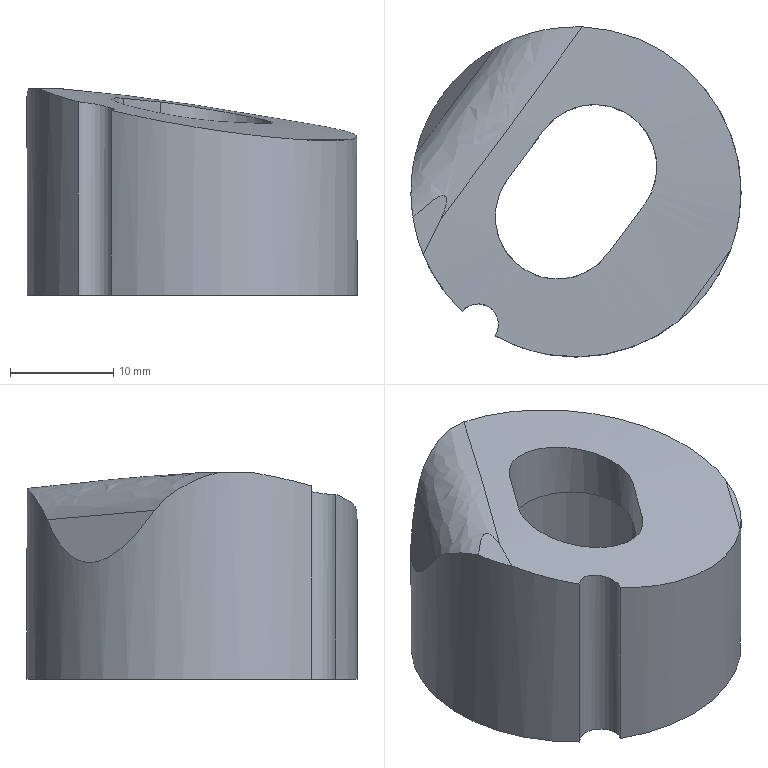Part | NX | features solid 2 | 1 solid | 14 faces | box 32.002 x 32 x 20.001 mm | volume 8892 mm3 | cylinder 5 | plane 5 | spline 4 | commonest cylinder face diameters 12.1 x2 4 x1 20.6 x1 32 x1
STEP:
#1=CARTESIAN_POINT('',(-895.514,283.241,15.738));
#2=VERTEX_POINT('',#1);
#3=CARTESIAN_POINT('',(-895.514,283.241,-3.));
#4=VERTEX_POINT('',#3);
#5=CARTESIAN_POINT('',(-895.514,283.241,7.));
#6=DIRECTION('',(0.,0.,1.));
#7=VECTOR('',#6,1000.);
#8=LINE('',#5,#7);
#9=EDGE_CURVE('',#2,#4,#8,.F.);
#10=ORIENTED_EDGE('',*,*,#9,.F.);
#11=CARTESIAN_POINT('',(-899.271,288.74,17.));
#12=VERTEX_POINT('',#11);
#13=CARTESIAN_POINT('',(-895.514,283.241,15.738));
#14=CARTESIAN_POINT('',(-897.14,284.792,16.198));
#15=CARTESIAN_POINT('',(-898.411,286.646,16.631));
#16=CARTESIAN_POINT('',(-899.271,288.74,17.));
#17=B_SPLINE_CURVE_WITH_KNOTS('',3,(#13,#14,#15,#16),.UNSPECIFIED.,.F.,.F.,(4,4),(0.,0.006783),.UNSPECIFIED.);
#18=EDGE_CURVE('',#2,#12,#17,.T.);
#19=ORIENTED_EDGE('',*,*,#18,.T.);
#20=CARTESIAN_POINT('',(-900.283,292.372,17.));
#21=VERTEX_POINT('',#20);
#22=CARTESIAN_POINT('',(-884.471,294.82,17.));
#23=DIRECTION('',(0.,0.,1.));
#24=DIRECTION('',(0.8041,-0.5945,0.));
#25=AXIS2_PLACEMENT_3D('',#22,#23,#24);
#26=CIRCLE('',#25,16.);
#27=EDGE_CURVE('',#21,#12,#26,.T.);
#28=ORIENTED_EDGE('',*,*,#27,.F.);
#29=CARTESIAN_POINT('',(-900.054,298.451,13.363));
#30=VERTEX_POINT('',#29);
#31=CARTESIAN_POINT('',(-900.054,298.451,13.364));
#32=CARTESIAN_POINT('',(-900.215,297.759,14.364));
#33=CARTESIAN_POINT('',(-900.552,295.786,15.797));
#34=CARTESIAN_POINT('',(-900.465,293.548,16.738));
#35=CARTESIAN_POINT('',(-900.283,292.372,17.));
#36=B_SPLINE_CURVE_WITH_KNOTS('',3,(#31,#32,#33,#34,#35),.UNSPECIFIED.,.F.,.F.,(4,1,4),(0.00005291,0.003662,0.007271),.UNSPECIFIED.);
#37=EDGE_CURVE('',#30,#21,#36,.T.);
#38=ORIENTED_EDGE('',*,*,#37,.F.);
#39=CARTESIAN_POINT('',(-892.21,308.824,12.452));
#40=VERTEX_POINT('',#39);
#41=CARTESIAN_POINT('',(-900.054,298.451,13.363));
#42=CARTESIAN_POINT('',(-899.869,299.241,12.221));
#43=CARTESIAN_POINT('',(-899.479,300.535,10.576));
#44=CARTESIAN_POINT('',(-898.519,302.555,8.915));
#45=CARTESIAN_POINT('',(-897.43,304.286,8.182));
#46=CARTESIAN_POINT('',(-896.043,305.932,8.408));
#47=CARTESIAN_POINT('',(-894.185,307.627,9.769));
#48=CARTESIAN_POINT('',(-892.968,308.405,11.341));
#49=CARTESIAN_POINT('',(-892.211,308.823,12.451));
#50=B_SPLINE_CURVE_WITH_KNOTS('',3,(#41,#42,#43,#44,#45,#46,#47,#48,#49),.UNSPECIFIED.,.F.,.F.,(4,1,1,1,1,1,4),(0.0003814,0.004577,0.006675,0.008773,0.01087,0.01297,0.01717),.UNSPECIFIED.);
#51=EDGE_CURVE('',#30,#40,#50,.T.);
#52=ORIENTED_EDGE('',*,*,#51,.T.);
#53=CARTESIAN_POINT('',(-883.852,310.808,15.384));
#54=VERTEX_POINT('',#53);
#55=CARTESIAN_POINT('',(-883.852,310.808,15.384));
#56=CARTESIAN_POINT('',(-885.432,310.869,15.657));
#57=CARTESIAN_POINT('',(-887.844,310.587,15.322));
#58=CARTESIAN_POINT('',(-890.602,309.649,14.029));
#59=CARTESIAN_POINT('',(-891.777,309.063,13.086));
#60=CARTESIAN_POINT('',(-892.209,308.824,12.452));
#61=B_SPLINE_CURVE_WITH_KNOTS('',3,(#55,#56,#57,#58,#59,#60),.UNSPECIFIED.,.F.,.F.,(4,1,1,4),(0.,0.00474,0.00711,0.00948),.UNSPECIFIED.);
#62=EDGE_CURVE('',#54,#40,#61,.T.);
#63=ORIENTED_EDGE('',*,*,#62,.F.);
#64=CARTESIAN_POINT('',(-869.466,289.266,12.058));
#65=VERTEX_POINT('',#64);
#66=CARTESIAN_POINT('',(-883.852,310.808,15.384));
#67=CARTESIAN_POINT('',(-881.365,310.711,14.956));
#68=CARTESIAN_POINT('',(-876.4,309.327,14.152));
#69=CARTESIAN_POINT('',(-870.701,304.091,13.225));
#70=CARTESIAN_POINT('',(-867.983,296.826,12.487));
#71=CARTESIAN_POINT('',(-868.587,291.647,12.148));
#72=CARTESIAN_POINT('',(-869.462,289.277,12.058));
#73=B_SPLINE_CURVE_WITH_KNOTS('',3,(#66,#67,#68,#69,#70,#71,#72),.UNSPECIFIED.,.F.,.F.,(4,1,1,1,4),(0.009525,0.01708,0.02464,0.03219,0.03975),.UNSPECIFIED.);
#74=EDGE_CURVE('',#54,#65,#73,.T.);
#75=ORIENTED_EDGE('',*,*,#74,.T.);
#76=CARTESIAN_POINT('',(-874.478,282.324,12.119));
#77=VERTEX_POINT('',#76);
#78=CARTESIAN_POINT('',(-869.467,289.262,12.058));
#79=CARTESIAN_POINT('',(-869.972,287.899,12.006));
#80=CARTESIAN_POINT('',(-871.325,285.364,11.905));
#81=CARTESIAN_POINT('',(-873.341,283.234,12.04));
#82=CARTESIAN_POINT('',(-874.475,282.327,12.118));
#83=B_SPLINE_CURVE_WITH_KNOTS('',3,(#78,#79,#80,#81,#82),.UNSPECIFIED.,.F.,.F.,(4,1,4),(0.,0.004301,0.008602),.UNSPECIFIED.);
#84=EDGE_CURVE('',#65,#77,#83,.T.);
#85=ORIENTED_EDGE('',*,*,#84,.T.);
#86=CARTESIAN_POINT('',(-892.304,280.868,14.91));
#87=VERTEX_POINT('',#86);
#88=CARTESIAN_POINT('',(-874.486,282.318,12.119));
#89=CARTESIAN_POINT('',(-876.987,280.32,12.293));
#90=CARTESIAN_POINT('',(-883.164,277.916,13.01));
#91=CARTESIAN_POINT('',(-889.551,279.322,14.258));
#92=CARTESIAN_POINT('',(-892.304,280.868,14.91));
#93=B_SPLINE_CURVE_WITH_KNOTS('',3,(#88,#89,#90,#91,#92),.UNSPECIFIED.,.F.,.F.,(4,1,4),(0.0484,0.05794,0.06748),.UNSPECIFIED.);
#94=EDGE_CURVE('',#77,#87,#93,.T.);
#95=ORIENTED_EDGE('',*,*,#94,.T.);
#96=CARTESIAN_POINT('',(-892.304,280.868,-3.));
#97=VERTEX_POINT('',#96);
#98=CARTESIAN_POINT('',(-892.304,280.868,7.));
#99=DIRECTION('',(0.,0.,1.));
#100=VECTOR('',#99,1000.);
#101=LINE('',#98,#100);
#102=EDGE_CURVE('',#97,#87,#101,.T.);
#103=ORIENTED_EDGE('',*,*,#102,.F.);
#104=CARTESIAN_POINT('',(-884.471,294.82,-3.));
#105=DIRECTION('',(0.,0.,1.));
#106=DIRECTION('',(0.8041,-0.5945,0.));
#107=AXIS2_PLACEMENT_3D('',#104,#105,#106);
#108=CIRCLE('',#107,16.);
#109=EDGE_CURVE('',#97,#4,#108,.T.);
#110=ORIENTED_EDGE('',*,*,#109,.T.);
#111=EDGE_LOOP('',(#10,#19,#28,#38,#52,#63,#75,#85,#95,#103,#110));
#112=FACE_BOUND('',#111,.T.);
#113=CARTESIAN_POINT('',(-884.471,294.82,-3.));
#114=DIRECTION('',(0.,0.,1.));
#115=DIRECTION('',(0.8041,-0.5945,0.));
#116=AXIS2_PLACEMENT_3D('',#113,#114,#115);
#117=CYLINDRICAL_SURFACE('',#116,16.);
#118=ADVANCED_FACE('',(#112),#117,.T.);
#119=CARTESIAN_POINT('',(-895.514,283.241,15.738));
#120=CARTESIAN_POINT('',(-895.184,283.634,15.721));
#121=CARTESIAN_POINT('',(-894.229,284.136,15.601));
#122=CARTESIAN_POINT('',(-892.684,283.722,15.28));
#123=CARTESIAN_POINT('',(-891.825,282.366,14.986));
#124=CARTESIAN_POINT('',(-892.025,281.299,14.908));
#125=CARTESIAN_POINT('',(-892.304,280.868,14.91));
#126=B_SPLINE_CURVE_WITH_KNOTS('',3,(#119,#120,#121,#122,#123,#124,#125),.UNSPECIFIED.,.F.,.F.,(4,1,1,1,4),(0.,0.001518,0.003036,0.004553,0.006071),.UNSPECIFIED.);
#127=EDGE_CURVE('',#2,#87,#126,.T.);
#128=ORIENTED_EDGE('',*,*,#127,.F.);
#129=ORIENTED_EDGE('',*,*,#9,.T.);
#130=CARTESIAN_POINT('',(-893.984,281.954,-3.));
#131=DIRECTION('',(0.,0.,1.));
#132=DIRECTION('',(-0.5945,-0.8041,0.));
#133=AXIS2_PLACEMENT_3D('',#130,#131,#132);
#134=CIRCLE('',#133,2.);
#135=EDGE_CURVE('',#97,#4,#134,.T.);
#136=ORIENTED_EDGE('',*,*,#135,.F.);
#137=ORIENTED_EDGE('',*,*,#102,.T.);
#138=EDGE_LOOP('',(#128,#129,#136,#137));
#139=FACE_BOUND('',#138,.T.);
#140=CARTESIAN_POINT('',(-893.984,281.954,-3.));
#141=DIRECTION('',(0.,0.,1.));
#142=DIRECTION('',(-0.5945,-0.8041,0.));
#143=AXIS2_PLACEMENT_3D('',#140,#141,#142);
#144=CYLINDRICAL_SURFACE('',#143,2.);
#145=ADVANCED_FACE('',(#139),#144,.F.);
#146=CARTESIAN_POINT('',(-891.119,296.004,16.081));
#147=VERTEX_POINT('',#146);
#148=CARTESIAN_POINT('',(-887.552,300.829,15.719));
#149=VERTEX_POINT('',#148);
#150=CARTESIAN_POINT('',(-891.119,296.004,16.081));
#151=CARTESIAN_POINT('',(-889.93,297.613,15.973));
#152=CARTESIAN_POINT('',(-888.741,299.221,15.851));
#153=CARTESIAN_POINT('',(-887.552,300.829,15.719));
#154=B_SPLINE_CURVE_WITH_KNOTS('',3,(#150,#151,#152,#153),.UNSPECIFIED.,.F.,.F.,(4,4),(0.,0.006011),.UNSPECIFIED.);
#155=EDGE_CURVE('',#147,#149,#154,.T.);
#156=ORIENTED_EDGE('',*,*,#155,.F.);
#157=CARTESIAN_POINT('',(-891.119,296.004,9.));
#158=VERTEX_POINT('',#157);
#159=CARTESIAN_POINT('',(-891.119,296.004,-3.));
#160=DIRECTION('',(0.,0.,1.));
#161=VECTOR('',#160,1000.);
#162=LINE('',#159,#161);
#163=EDGE_CURVE('',#158,#147,#162,.T.);
#164=ORIENTED_EDGE('',*,*,#163,.F.);
#165=CARTESIAN_POINT('',(-887.552,300.829,9.));
#166=VERTEX_POINT('',#165);
#167=CARTESIAN_POINT('',(-889.336,298.416,9.));
#168=DIRECTION('',(-0.5945,-0.8041,0.));
#169=VECTOR('',#168,1000.);
#170=LINE('',#167,#169);
#171=EDGE_CURVE('',#166,#158,#170,.T.);
#172=ORIENTED_EDGE('',*,*,#171,.F.);
#173=CARTESIAN_POINT('',(-887.552,300.829,-3.));
#174=DIRECTION('',(0.,0.,1.));
#175=VECTOR('',#174,1000.);
#176=LINE('',#173,#175);
#177=EDGE_CURVE('',#166,#149,#176,.T.);
#178=ORIENTED_EDGE('',*,*,#177,.T.);
#179=EDGE_LOOP('',(#156,#164,#172,#178));
#180=FACE_BOUND('',#179,.T.);
#181=CARTESIAN_POINT('',(-887.552,300.829,-3.));
#182=DIRECTION('',(-0.8041,0.5945,0.));
#183=DIRECTION('',(0.,0.,1.));
#184=AXIS2_PLACEMENT_3D('',#181,#182,#183);
#185=PLANE('',#184);
#186=ADVANCED_FACE('',(#180),#185,.F.);
#187=CARTESIAN_POINT('',(-881.39,288.81,13.806));
#188=VERTEX_POINT('',#187);
#189=CARTESIAN_POINT('',(-888.385,286.745,14.817));
#190=VERTEX_POINT('',#189);
#191=CARTESIAN_POINT('',(-881.39,288.81,13.806));
#192=CARTESIAN_POINT('',(-882.181,287.741,13.844));
#193=CARTESIAN_POINT('',(-884.447,286.183,14.078));
#194=CARTESIAN_POINT('',(-887.172,286.288,14.56));
#195=CARTESIAN_POINT('',(-888.385,286.745,14.817));
#196=B_SPLINE_CURVE_WITH_KNOTS('',3,(#191,#192,#193,#194,#195),.UNSPECIFIED.,.F.,.F.,(4,1,4),(0.,0.003933,0.007866),.UNSPECIFIED.);
#197=EDGE_CURVE('',#188,#190,#196,.T.);
#198=ORIENTED_EDGE('',*,*,#197,.F.);
#199=CARTESIAN_POINT('',(-881.39,288.81,9.));
#200=VERTEX_POINT('',#199);
#201=CARTESIAN_POINT('',(-881.39,288.81,-3.));
#202=DIRECTION('',(0.,0.,1.));
#203=VECTOR('',#202,1000.);
#204=LINE('',#201,#203);
#205=EDGE_CURVE('',#200,#188,#204,.T.);
#206=ORIENTED_EDGE('',*,*,#205,.F.);
#207=CARTESIAN_POINT('',(-886.255,292.407,9.));
#208=DIRECTION('',(0.,0.,1.));
#209=DIRECTION('',(0.8041,-0.5945,0.));
#210=AXIS2_PLACEMENT_3D('',#207,#208,#209);
#211=CIRCLE('',#210,6.05);
#212=EDGE_CURVE('',#158,#200,#211,.T.);
#213=ORIENTED_EDGE('',*,*,#212,.F.);
#214=ORIENTED_EDGE('',*,*,#163,.T.);
#215=CARTESIAN_POINT('',(-892.001,290.513,15.811));
#216=VERTEX_POINT('',#215);
#217=CARTESIAN_POINT('',(-892.001,290.513,15.811));
#218=CARTESIAN_POINT('',(-892.596,292.318,16.078));
#219=CARTESIAN_POINT('',(-892.277,294.439,16.187));
#220=CARTESIAN_POINT('',(-891.119,296.004,16.081));
#221=B_SPLINE_CURVE_WITH_KNOTS('',3,(#217,#218,#219,#220),.UNSPECIFIED.,.F.,.F.,(4,4),(0.01333,0.0191),.UNSPECIFIED.);
#222=EDGE_CURVE('',#216,#147,#221,.T.);
#223=ORIENTED_EDGE('',*,*,#222,.F.);
#224=CARTESIAN_POINT('',(-888.385,286.745,14.817));
#225=CARTESIAN_POINT('',(-889.1,287.014,14.968));
#226=CARTESIAN_POINT('',(-890.195,287.727,15.223));
#227=CARTESIAN_POINT('',(-890.817,288.423,15.404));
#228=CARTESIAN_POINT('',(-891.055,288.723,15.477));
#229=CARTESIAN_POINT('',(-891.141,288.839,15.504));
#230=CARTESIAN_POINT('',(-891.167,288.875,15.512));
#231=CARTESIAN_POINT('',(-891.286,289.044,15.549));
#232=CARTESIAN_POINT('',(-891.522,289.414,15.626));
#233=CARTESIAN_POINT('',(-891.778,289.91,15.717));
#234=CARTESIAN_POINT('',(-891.935,290.315,15.781));
#235=CARTESIAN_POINT('',(-892.001,290.513,15.811));
#236=B_SPLINE_CURVE_WITH_KNOTS('',3,(#224,#225,#226,#227,#228,#229,#230,#231,#232,#233,#234,#235),.UNSPECIFIED.,.F.,.F.,(4,1,1,1,1,1,1,1,1,4),(0.,0.25,0.5,0.5625,0.625,0.6562,0.6875,0.75,0.875,1.),.UNSPECIFIED.);
#237=EDGE_CURVE('',#190,#216,#236,.T.);
#238=ORIENTED_EDGE('',*,*,#237,.F.);
#239=EDGE_LOOP('',(#198,#206,#213,#214,#223,#238));
#240=FACE_BOUND('',#239,.T.);
#241=CARTESIAN_POINT('',(-886.255,292.407,-3.));
#242=DIRECTION('',(0.,0.,1.));
#243=DIRECTION('',(0.8041,-0.5945,0.));
#244=AXIS2_PLACEMENT_3D('',#241,#242,#243);
#245=CYLINDRICAL_SURFACE('',#244,6.05);
#246=ADVANCED_FACE('',(#240),#245,.F.);
#247=ORIENTED_EDGE('',*,*,#205,.T.);
#248=CARTESIAN_POINT('',(-877.823,293.635,13.62));
#249=VERTEX_POINT('',#248);
#250=CARTESIAN_POINT('',(-881.39,288.81,13.806));
#251=CARTESIAN_POINT('',(-880.201,290.419,13.749));
#252=CARTESIAN_POINT('',(-879.012,292.027,13.687));
#253=CARTESIAN_POINT('',(-877.823,293.635,13.62));
#254=B_SPLINE_CURVE_WITH_KNOTS('',3,(#250,#251,#252,#253),.UNSPECIFIED.,.F.,.F.,(4,4),(0.,0.006003),.UNSPECIFIED.);
#255=EDGE_CURVE('',#188,#249,#254,.T.);
#256=ORIENTED_EDGE('',*,*,#255,.T.);
#257=CARTESIAN_POINT('',(-877.823,293.635,9.));
#258=VERTEX_POINT('',#257);
#259=CARTESIAN_POINT('',(-877.823,293.635,-3.));
#260=DIRECTION('',(0.,0.,1.));
#261=VECTOR('',#260,1000.);
#262=LINE('',#259,#261);
#263=EDGE_CURVE('',#258,#249,#262,.T.);
#264=ORIENTED_EDGE('',*,*,#263,.F.);
#265=CARTESIAN_POINT('',(-879.607,291.223,9.));
#266=DIRECTION('',(-0.5945,-0.8041,0.));
#267=VECTOR('',#266,1000.);
#268=LINE('',#265,#267);
#269=EDGE_CURVE('',#258,#200,#268,.T.);
#270=ORIENTED_EDGE('',*,*,#269,.T.);
#271=EDGE_LOOP('',(#247,#256,#264,#270));
#272=FACE_BOUND('',#271,.T.);
#273=CARTESIAN_POINT('',(-877.823,293.635,-3.));
#274=DIRECTION('',(-0.8041,0.5945,0.));
#275=DIRECTION('',(0.,0.,1.));
#276=AXIS2_PLACEMENT_3D('',#273,#274,#275);
#277=PLANE('',#276);
#278=ADVANCED_FACE('',(#272),#277,.T.);
#279=CARTESIAN_POINT('',(-880.292,302.786,14.561));
#280=VERTEX_POINT('',#279);
#281=CARTESIAN_POINT('',(-887.552,300.829,15.719));
#282=CARTESIAN_POINT('',(-886.733,301.936,15.628));
#283=CARTESIAN_POINT('',(-884.362,303.523,15.27));
#284=CARTESIAN_POINT('',(-881.539,303.325,14.787));
#285=CARTESIAN_POINT('',(-880.291,302.787,14.561));
#286=B_SPLINE_CURVE_WITH_KNOTS('',3,(#281,#282,#283,#284,#285),.UNSPECIFIED.,.F.,.F.,(4,1,4),(0.,0.004081,0.008162),.UNSPECIFIED.);
#287=EDGE_CURVE('',#149,#280,#286,.T.);
#288=ORIENTED_EDGE('',*,*,#287,.F.);
#289=ORIENTED_EDGE('',*,*,#177,.F.);
#290=CARTESIAN_POINT('',(-882.688,297.232,9.));
#291=DIRECTION('',(0.,0.,1.));
#292=DIRECTION('',(0.8041,-0.5945,0.));
#293=AXIS2_PLACEMENT_3D('',#290,#291,#292);
#294=CIRCLE('',#293,6.05);
#295=EDGE_CURVE('',#258,#166,#294,.T.);
#296=ORIENTED_EDGE('',*,*,#295,.F.);
#297=ORIENTED_EDGE('',*,*,#263,.T.);
#298=CARTESIAN_POINT('',(-877.689,300.655,14.044));
#299=VERTEX_POINT('',#298);
#300=CARTESIAN_POINT('',(-877.696,300.65,14.045));
#301=CARTESIAN_POINT('',(-876.999,299.632,13.884));
#302=CARTESIAN_POINT('',(-876.241,297.124,13.625));
#303=CARTESIAN_POINT('',(-877.073,294.649,13.578));
#304=CARTESIAN_POINT('',(-877.823,293.635,13.62));
#305=B_SPLINE_CURVE_WITH_KNOTS('',3,(#300,#301,#302,#303,#304),.UNSPECIFIED.,.F.,.F.,(4,1,4),(0.01159,0.01532,0.01906),.UNSPECIFIED.);
#306=EDGE_CURVE('',#299,#249,#305,.T.);
#307=ORIENTED_EDGE('',*,*,#306,.F.);
#308=CARTESIAN_POINT('',(-880.291,302.787,14.561));
#309=CARTESIAN_POINT('',(-879.102,302.274,14.345));
#310=CARTESIAN_POINT('',(-878.247,301.455,14.173));
#311=CARTESIAN_POINT('',(-877.696,300.65,14.045));
#312=B_SPLINE_CURVE_WITH_KNOTS('',3,(#308,#309,#310,#311),.UNSPECIFIED.,.F.,.F.,(4,4),(0.,1.),.UNSPECIFIED.);
#313=EDGE_CURVE('',#280,#299,#312,.T.);
#314=ORIENTED_EDGE('',*,*,#313,.F.);
#315=EDGE_LOOP('',(#288,#289,#296,#297,#307,#314));
#316=FACE_BOUND('',#315,.T.);
#317=CARTESIAN_POINT('',(-882.688,297.232,-3.));
#318=DIRECTION('',(0.,0.,1.));
#319=DIRECTION('',(0.8041,-0.5945,0.));
#320=AXIS2_PLACEMENT_3D('',#317,#318,#319);
#321=CYLINDRICAL_SURFACE('',#320,6.05);
#322=ADVANCED_FACE('',(#316),#321,.F.);
#323=CARTESIAN_POINT('',(-876.189,288.696,-3.));
#324=VERTEX_POINT('',#323);
#325=CARTESIAN_POINT('',(-884.471,294.82,-3.));
#326=DIRECTION('',(0.,0.,1.));
#327=DIRECTION('',(0.8041,-0.5945,0.));
#328=AXIS2_PLACEMENT_3D('',#325,#326,#327);
#329=CIRCLE('',#328,10.3);
#330=EDGE_CURVE('',#324,#324,#329,.T.);
#331=ORIENTED_EDGE('',*,*,#330,.T.);
#332=EDGE_LOOP('',(#331));
#333=FACE_BOUND('',#332,.T.);
#334=ORIENTED_EDGE('',*,*,#109,.F.);
#335=ORIENTED_EDGE('',*,*,#135,.T.);
#336=EDGE_LOOP('',(#334,#335));
#337=FACE_BOUND('',#336,.T.);
#338=CARTESIAN_POINT('',(-884.471,294.82,-3.));
#339=DIRECTION('',(0.,0.,1.));
#340=DIRECTION('',(0.8041,-0.5945,0.));
#341=AXIS2_PLACEMENT_3D('',#338,#339,#340);
#342=PLANE('',#341);
#343=ADVANCED_FACE('',(#333,#337),#342,.F.);
#344=CARTESIAN_POINT('',(-897.597,292.138,17.));
#345=VERTEX_POINT('',#344);
#346=CARTESIAN_POINT('',(-900.283,292.372,17.));
#347=CARTESIAN_POINT('',(-899.906,292.726,17.));
#348=CARTESIAN_POINT('',(-899.329,293.246,17.));
#349=CARTESIAN_POINT('',(-898.514,293.889,17.));
#350=CARTESIAN_POINT('',(-897.967,294.237,17.));
#351=CARTESIAN_POINT('',(-897.497,294.458,17.));
#352=CARTESIAN_POINT('',(-897.042,294.425,17.));
#353=CARTESIAN_POINT('',(-896.984,293.97,17.));
#354=CARTESIAN_POINT('',(-897.075,293.471,17.));
#355=CARTESIAN_POINT('',(-897.282,292.85,17.));
#356=CARTESIAN_POINT('',(-897.488,292.374,17.));
#357=CARTESIAN_POINT('',(-897.597,292.137,17.));
#358=B_SPLINE_CURVE_WITH_KNOTS('',3,(#346,#347,#348,#349,#350,#351,#352,#353,#354,#355,#356,#357),.UNSPECIFIED.,.F.,.F.,(4,1,1,1,1,1,1,1,1,4),(0.004738,0.006289,0.007064,0.00784,0.008227,0.008615,0.009003,0.00939,0.01017,0.01094),.UNSPECIFIED.);
#359=EDGE_CURVE('',#21,#345,#358,.T.);
#360=ORIENTED_EDGE('',*,*,#359,.F.);
#361=ORIENTED_EDGE('',*,*,#27,.T.);
#362=CARTESIAN_POINT('',(-899.271,288.74,17.));
#363=CARTESIAN_POINT('',(-898.681,289.86,17.));
#364=CARTESIAN_POINT('',(-898.122,290.992,17.));
#365=CARTESIAN_POINT('',(-897.597,292.137,17.));
#366=B_SPLINE_CURVE_WITH_KNOTS('',3,(#362,#363,#364,#365),.UNSPECIFIED.,.F.,.F.,(4,4),(0.002381,0.006155),.UNSPECIFIED.);
#367=EDGE_CURVE('',#12,#345,#366,.T.);
#368=ORIENTED_EDGE('',*,*,#367,.T.);
#369=EDGE_LOOP('',(#360,#361,#368));
#370=FACE_BOUND('',#369,.T.);
#371=CARTESIAN_POINT('',(-884.471,294.82,17.));
#372=DIRECTION('',(0.,0.,1.));
#373=DIRECTION('',(0.8041,-0.5945,0.));
#374=AXIS2_PLACEMENT_3D('',#371,#372,#373);
#375=PLANE('',#374);
#376=ADVANCED_FACE('',(#370),#375,.T.);
#377=ORIENTED_EDGE('',*,*,#330,.F.);
#378=EDGE_LOOP('',(#377));
#379=FACE_BOUND('',#378,.T.);
#380=CARTESIAN_POINT('',(-876.189,288.696,9.));
#381=VERTEX_POINT('',#380);
#382=CARTESIAN_POINT('',(-884.471,294.82,9.));
#383=DIRECTION('',(0.,0.,1.));
#384=DIRECTION('',(0.8041,-0.5945,0.));
#385=AXIS2_PLACEMENT_3D('',#382,#383,#384);
#386=CIRCLE('',#385,10.3);
#387=EDGE_CURVE('',#381,#381,#386,.T.);
#388=ORIENTED_EDGE('',*,*,#387,.T.);
#389=EDGE_LOOP('',(#388));
#390=FACE_BOUND('',#389,.T.);
#391=CARTESIAN_POINT('',(-884.471,294.82,-3.));
#392=DIRECTION('',(0.,0.,1.));
#393=DIRECTION('',(0.8041,-0.5945,0.));
#394=AXIS2_PLACEMENT_3D('',#391,#392,#393);
#395=CYLINDRICAL_SURFACE('',#394,10.3);
#396=ADVANCED_FACE('',(#379,#390),#395,.F.);
#397=ORIENTED_EDGE('',*,*,#295,.T.);
#398=ORIENTED_EDGE('',*,*,#171,.T.);
#399=ORIENTED_EDGE('',*,*,#212,.T.);
#400=ORIENTED_EDGE('',*,*,#269,.F.);
#401=EDGE_LOOP('',(#397,#398,#399,#400));
#402=FACE_BOUND('',#401,.T.);
#403=ORIENTED_EDGE('',*,*,#387,.F.);
#404=EDGE_LOOP('',(#403));
#405=FACE_BOUND('',#404,.T.);
#406=CARTESIAN_POINT('',(-884.471,294.82,9.));
#407=DIRECTION('',(0.,0.,1.));
#408=DIRECTION('',(0.8041,-0.5945,0.));
#409=AXIS2_PLACEMENT_3D('',#406,#407,#408);
#410=PLANE('',#409);
#411=ADVANCED_FACE('',(#402,#405),#410,.F.);
#412=CARTESIAN_POINT('',(-883.852,310.808,15.384));
#413=CARTESIAN_POINT('',(-885.189,308.954,15.592));
#414=CARTESIAN_POINT('',(-887.153,306.246,15.878));
#415=CARTESIAN_POINT('',(-889.687,302.779,16.209));
#416=CARTESIAN_POINT('',(-891.545,300.252,16.431));
#417=CARTESIAN_POINT('',(-893.061,298.203,16.595));
#418=CARTESIAN_POINT('',(-894.246,296.608,16.713));
#419=CARTESIAN_POINT('',(-894.993,295.607,16.783));
#420=CARTESIAN_POINT('',(-895.55,294.861,16.833));
#421=CARTESIAN_POINT('',(-895.976,294.292,16.87));
#422=CARTESIAN_POINT('',(-896.094,294.135,16.88));
#423=CARTESIAN_POINT('',(-896.257,293.917,16.894));
#424=CARTESIAN_POINT('',(-896.538,293.544,16.917));
#425=CARTESIAN_POINT('',(-896.989,292.946,16.954));
#426=CARTESIAN_POINT('',(-897.389,292.418,16.985));
#427=CARTESIAN_POINT('',(-897.6,292.14,17.001));
#428=B_SPLINE_CURVE_WITH_KNOTS('',3,(#412,#413,#414,#415,#416,#417,#418,#419,#420,#421,#422,#423,#424,#425,#426,#427),.UNSPECIFIED.,.F.,.F.,(4,1,1,1,1,1,1,1,1,1,1,1,1,4),(0.3861,0.4212,0.4388,0.4563,0.4739,0.4827,0.4915,0.4959,0.5003,0.5025,0.5047,0.5091,0.5178,0.5266),.UNSPECIFIED.);
#429=EDGE_CURVE('',#54,#345,#428,.T.);
#430=ORIENTED_EDGE('',*,*,#429,.T.);
#431=ORIENTED_EDGE('',*,*,#367,.F.);
#432=ORIENTED_EDGE('',*,*,#18,.F.);
#433=ORIENTED_EDGE('',*,*,#127,.T.);
#434=ORIENTED_EDGE('',*,*,#94,.F.);
#435=CARTESIAN_POINT('',(-874.482,282.323,12.119));
#436=CARTESIAN_POINT('',(-872.815,284.62,12.099));
#437=CARTESIAN_POINT('',(-871.143,286.936,12.078));
#438=CARTESIAN_POINT('',(-869.466,289.271,12.058));
#439=B_SPLINE_CURVE_WITH_KNOTS('',3,(#435,#436,#437,#438),.UNSPECIFIED.,.F.,.F.,(4,4),(0.8352,0.9009),.UNSPECIFIED.);
#440=EDGE_CURVE('',#77,#65,#439,.T.);
#441=ORIENTED_EDGE('',*,*,#440,.T.);
#442=ORIENTED_EDGE('',*,*,#74,.F.);
#443=EDGE_LOOP('',(#430,#431,#432,#433,#434,#441,#442));
#444=FACE_BOUND('',#443,.T.);
#445=ORIENTED_EDGE('',*,*,#287,.T.);
#446=ORIENTED_EDGE('',*,*,#313,.T.);
#447=ORIENTED_EDGE('',*,*,#306,.T.);
#448=ORIENTED_EDGE('',*,*,#255,.F.);
#449=ORIENTED_EDGE('',*,*,#197,.T.);
#450=ORIENTED_EDGE('',*,*,#237,.T.);
#451=ORIENTED_EDGE('',*,*,#222,.T.);
#452=ORIENTED_EDGE('',*,*,#155,.T.);
#453=EDGE_LOOP('',(#445,#446,#447,#448,#449,#450,#451,#452));
#454=FACE_BOUND('',#453,.T.);
#455=CARTESIAN_POINT('',(-881.127,272.651,12.127));
#456=CARTESIAN_POINT('',(-882.862,273.89,12.543));
#457=CARTESIAN_POINT('',(-884.597,275.129,12.964));
#458=CARTESIAN_POINT('',(-886.332,276.368,13.389));
#459=CARTESIAN_POINT('',(-890.379,279.257,14.393));
#460=CARTESIAN_POINT('',(-894.424,282.146,15.42));
#461=CARTESIAN_POINT('',(-896.735,283.796,16.015));
#462=CARTESIAN_POINT('',(-899.045,285.446,16.616));
#463=CARTESIAN_POINT('',(-901.355,287.095,17.222));
#464=CARTESIAN_POINT('',(-881.025,272.794,12.127));
#465=CARTESIAN_POINT('',(-882.76,274.033,12.542));
#466=CARTESIAN_POINT('',(-884.496,275.272,12.963));
#467=CARTESIAN_POINT('',(-886.23,276.51,13.388));
#468=CARTESIAN_POINT('',(-890.277,279.4,14.391));
#469=CARTESIAN_POINT('',(-894.323,282.288,15.417));
#470=CARTESIAN_POINT('',(-896.633,283.939,16.012));
#471=CARTESIAN_POINT('',(-898.944,285.588,16.613));
#472=CARTESIAN_POINT('',(-901.254,287.238,17.218));
#473=CARTESIAN_POINT('',(-880.923,272.936,12.126));
#474=CARTESIAN_POINT('',(-882.659,274.175,12.542));
#475=CARTESIAN_POINT('',(-884.394,275.414,12.962));
#476=CARTESIAN_POINT('',(-886.129,276.653,13.386));
#477=CARTESIAN_POINT('',(-890.176,279.543,14.389));
#478=CARTESIAN_POINT('',(-894.221,282.431,15.415));
#479=CARTESIAN_POINT('',(-896.532,284.081,16.008));
#480=CARTESIAN_POINT('',(-898.842,285.731,16.609));
#481=CARTESIAN_POINT('',(-901.152,287.381,17.214));
#482=CARTESIAN_POINT('',(-880.822,273.079,12.126));
#483=CARTESIAN_POINT('',(-882.557,274.318,12.541));
#484=CARTESIAN_POINT('',(-884.293,275.557,12.961));
#485=CARTESIAN_POINT('',(-886.027,276.795,13.385));
#486=CARTESIAN_POINT('',(-890.075,279.685,14.386));
#487=CARTESIAN_POINT('',(-894.12,282.574,15.412));
#488=CARTESIAN_POINT('',(-896.431,284.224,16.005));
#489=CARTESIAN_POINT('',(-898.741,285.874,16.606));
#490=CARTESIAN_POINT('',(-901.051,287.523,17.21));
#491=CARTESIAN_POINT('',(-879.472,274.972,12.121));
#492=CARTESIAN_POINT('',(-881.208,276.211,12.531));
#493=CARTESIAN_POINT('',(-882.944,277.451,12.946));
#494=CARTESIAN_POINT('',(-884.679,278.689,13.366));
#495=CARTESIAN_POINT('',(-888.727,281.58,14.357));
#496=CARTESIAN_POINT('',(-892.773,284.469,15.373));
#497=CARTESIAN_POINT('',(-895.084,286.119,15.962));
#498=CARTESIAN_POINT('',(-897.395,287.769,16.557));
#499=CARTESIAN_POINT('',(-899.706,289.419,17.155));
#500=CARTESIAN_POINT('',(-878.123,276.865,12.114));
#501=CARTESIAN_POINT('',(-879.859,278.105,12.517));
#502=CARTESIAN_POINT('',(-881.595,279.344,12.927));
#503=CARTESIAN_POINT('',(-883.331,280.584,13.341));
#504=CARTESIAN_POINT('',(-887.38,283.475,14.32));
#505=CARTESIAN_POINT('',(-891.427,286.364,15.324));
#506=CARTESIAN_POINT('',(-893.739,288.015,15.906));
#507=CARTESIAN_POINT('',(-896.05,289.666,16.492));
#508=CARTESIAN_POINT('',(-898.362,291.316,17.082));
#509=CARTESIAN_POINT('',(-876.875,278.616,12.105));
#510=CARTESIAN_POINT('',(-878.612,279.856,12.503));
#511=CARTESIAN_POINT('',(-880.349,281.096,12.905));
#512=CARTESIAN_POINT('',(-882.085,282.336,13.313));
#513=CARTESIAN_POINT('',(-886.135,285.227,14.278));
#514=CARTESIAN_POINT('',(-890.183,288.118,15.268));
#515=CARTESIAN_POINT('',(-892.496,289.769,15.84));
#516=CARTESIAN_POINT('',(-894.808,291.42,16.417));
#517=CARTESIAN_POINT('',(-897.12,293.071,16.999));
#518=CARTESIAN_POINT('',(-874.406,282.082,12.085));
#519=CARTESIAN_POINT('',(-876.144,283.323,12.467));
#520=CARTESIAN_POINT('',(-877.882,284.563,12.855));
#521=CARTESIAN_POINT('',(-879.62,285.804,13.249));
#522=CARTESIAN_POINT('',(-883.673,288.697,14.179));
#523=CARTESIAN_POINT('',(-887.724,291.589,15.134));
#524=CARTESIAN_POINT('',(-890.038,293.242,15.686));
#525=CARTESIAN_POINT('',(-892.352,294.894,16.242));
#526=CARTESIAN_POINT('',(-894.666,296.546,16.803));
#527=CARTESIAN_POINT('',(-871.937,285.547,12.061));
#528=CARTESIAN_POINT('',(-873.677,286.789,12.423));
#529=CARTESIAN_POINT('',(-875.416,288.031,12.792));
#530=CARTESIAN_POINT('',(-877.156,289.272,13.167));
#531=CARTESIAN_POINT('',(-881.212,292.168,14.052));
#532=CARTESIAN_POINT('',(-885.267,295.063,14.961));
#533=CARTESIAN_POINT('',(-887.584,296.717,15.486));
#534=CARTESIAN_POINT('',(-889.901,298.371,16.016));
#535=CARTESIAN_POINT('',(-892.216,300.024,16.55));
#536=CARTESIAN_POINT('',(-870.715,287.262,12.049));
#537=CARTESIAN_POINT('',(-872.456,288.505,12.401));
#538=CARTESIAN_POINT('',(-874.197,289.747,12.759));
#539=CARTESIAN_POINT('',(-875.937,290.989,13.122));
#540=CARTESIAN_POINT('',(-879.996,293.886,13.983));
#541=CARTESIAN_POINT('',(-884.053,296.782,14.866));
#542=CARTESIAN_POINT('',(-886.371,298.437,15.377));
#543=CARTESIAN_POINT('',(-888.688,300.091,15.892));
#544=CARTESIAN_POINT('',(-891.006,301.746,16.411));
#545=CARTESIAN_POINT('',(-868.306,290.645,12.025));
#546=CARTESIAN_POINT('',(-870.049,291.889,12.354));
#547=CARTESIAN_POINT('',(-871.791,293.132,12.689));
#548=CARTESIAN_POINT('',(-873.533,294.375,13.029));
#549=CARTESIAN_POINT('',(-877.597,297.276,13.834));
#550=CARTESIAN_POINT('',(-881.659,300.175,14.662));
#551=CARTESIAN_POINT('',(-883.979,301.831,15.142));
#552=CARTESIAN_POINT('',(-886.299,303.487,15.626));
#553=CARTESIAN_POINT('',(-888.619,305.143,16.113));
#554=CARTESIAN_POINT('',(-865.896,294.028,11.999));
#555=CARTESIAN_POINT('',(-867.641,295.273,12.302));
#556=CARTESIAN_POINT('',(-869.386,296.518,12.61));
#557=CARTESIAN_POINT('',(-871.13,297.762,12.924));
#558=CARTESIAN_POINT('',(-875.199,300.666,13.665));
#559=CARTESIAN_POINT('',(-879.267,303.569,14.429));
#560=CARTESIAN_POINT('',(-881.59,305.227,14.872));
#561=CARTESIAN_POINT('',(-883.914,306.885,15.319));
#562=CARTESIAN_POINT('',(-886.237,308.543,15.771));
#563=CARTESIAN_POINT('',(-864.708,295.696,11.987));
#564=CARTESIAN_POINT('',(-866.455,296.942,12.276));
#565=CARTESIAN_POINT('',(-868.2,298.187,12.57));
#566=CARTESIAN_POINT('',(-869.946,299.433,12.869));
#567=CARTESIAN_POINT('',(-874.018,302.338,13.577));
#568=CARTESIAN_POINT('',(-878.088,305.242,14.308));
#569=CARTESIAN_POINT('',(-880.413,306.902,14.731));
#570=CARTESIAN_POINT('',(-882.738,308.561,15.16));
#571=CARTESIAN_POINT('',(-885.063,310.22,15.592));
#572=CARTESIAN_POINT('',(-863.52,297.364,11.973));
#573=CARTESIAN_POINT('',(-865.268,298.61,12.248));
#574=CARTESIAN_POINT('',(-867.015,299.857,12.527));
#575=CARTESIAN_POINT('',(-868.762,301.103,12.811));
#576=CARTESIAN_POINT('',(-872.836,304.01,13.485));
#577=CARTESIAN_POINT('',(-876.909,306.917,14.181));
#578=CARTESIAN_POINT('',(-879.236,308.577,14.584));
#579=CARTESIAN_POINT('',(-881.563,310.237,14.992));
#580=CARTESIAN_POINT('',(-883.889,311.897,15.405));
#581=CARTESIAN_POINT('',(-862.332,299.032,11.959));
#582=CARTESIAN_POINT('',(-864.081,300.279,12.219));
#583=CARTESIAN_POINT('',(-865.829,301.526,12.483));
#584=CARTESIAN_POINT('',(-867.577,302.774,12.752));
#585=CARTESIAN_POINT('',(-871.655,305.683,13.39));
#586=CARTESIAN_POINT('',(-875.731,308.591,14.048));
#587=CARTESIAN_POINT('',(-878.06,310.252,14.43));
#588=CARTESIAN_POINT('',(-880.389,311.914,14.818));
#589=CARTESIAN_POINT('',(-882.717,313.575,15.209));
#590=B_SPLINE_SURFACE_WITH_KNOTS('',5,5,((#455,#456,#457,#458,#459,#460,#461,#462,#463),(#464,#465,#466,#467,#468,#469,#470,#471,#472),(#473,#474,#475,#476,#477,#478,#479,#480,#481),(#482,#483,#484,#485,#486,#487,#488,#489,#490),(#491,#492,#493,#494,#495,#496,#497,#498,#499),(#500,#501,#502,#503,#504,#505,#506,#507,#508),(#509,#510,#511,#512,#513,#514,#515,#516,#517),(#518,#519,#520,#521,#522,#523,#524,#525,#526),(#527,#528,#529,#530,#531,#532,#533,#534,#535),(#536,#537,#538,#539,#540,#541,#542,#543,#544),(#545,#546,#547,#548,#549,#550,#551,#552,#553),(#554,#555,#556,#557,#558,#559,#560,#561,#562),(#563,#564,#565,#566,#567,#568,#569,#570,#571),(#572,#573,#574,#575,#576,#577,#578,#579,#580),(#581,#582,#583,#584,#585,#586,#587,#588,#589)),.UNSPECIFIED.,.F.,.F.,.F.,(6,3,3,3,6),(6,3,6),(0.6499,0.6529,0.69,0.7264,0.7618),(0.3047,0.518,0.8025),.UNSPECIFIED.);
#591=ADVANCED_FACE('',(#444,#454),#590,.T.);
#592=ORIENTED_EDGE('',*,*,#440,.F.);
#593=ORIENTED_EDGE('',*,*,#84,.F.);
#594=EDGE_LOOP('',(#592,#593));
#595=FACE_BOUND('',#594,.T.);
#596=CARTESIAN_POINT('',(-869.433,289.31,12.057));
#597=CARTESIAN_POINT('',(-869.316,289.224,12.034));
#598=CARTESIAN_POINT('',(-869.199,289.138,12.007));
#599=CARTESIAN_POINT('',(-869.083,289.052,11.976));
#600=CARTESIAN_POINT('',(-868.968,288.968,11.941));
#601=CARTESIAN_POINT('',(-868.854,288.883,11.902));
#602=CARTESIAN_POINT('',(-869.853,288.725,12.062));
#603=CARTESIAN_POINT('',(-869.736,288.639,12.039));
#604=CARTESIAN_POINT('',(-869.619,288.553,12.012));
#605=CARTESIAN_POINT('',(-869.503,288.467,11.98));
#606=CARTESIAN_POINT('',(-869.388,288.383,11.945));
#607=CARTESIAN_POINT('',(-869.274,288.298,11.906));
#608=CARTESIAN_POINT('',(-870.273,288.14,12.067));
#609=CARTESIAN_POINT('',(-870.156,288.054,12.043));
#610=CARTESIAN_POINT('',(-870.04,287.968,12.016));
#611=CARTESIAN_POINT('',(-869.924,287.883,11.984));
#612=CARTESIAN_POINT('',(-869.809,287.798,11.949));
#613=CARTESIAN_POINT('',(-869.695,287.714,11.91));
#614=CARTESIAN_POINT('',(-870.694,287.555,12.072));
#615=CARTESIAN_POINT('',(-870.577,287.469,12.048));
#616=CARTESIAN_POINT('',(-870.461,287.383,12.02));
#617=CARTESIAN_POINT('',(-870.345,287.298,11.989));
#618=CARTESIAN_POINT('',(-870.23,287.213,11.953));
#619=CARTESIAN_POINT('',(-870.116,287.129,11.914));
#620=CARTESIAN_POINT('',(-871.707,286.148,12.084));
#621=CARTESIAN_POINT('',(-871.591,286.062,12.06));
#622=CARTESIAN_POINT('',(-871.475,285.977,12.031));
#623=CARTESIAN_POINT('',(-871.36,285.891,11.999));
#624=CARTESIAN_POINT('',(-871.245,285.807,11.963));
#625=CARTESIAN_POINT('',(-871.132,285.723,11.923));
#626=CARTESIAN_POINT('',(-872.723,284.743,12.097));
#627=CARTESIAN_POINT('',(-872.607,284.657,12.072));
#628=CARTESIAN_POINT('',(-872.491,284.571,12.043));
#629=CARTESIAN_POINT('',(-872.376,284.486,12.01));
#630=CARTESIAN_POINT('',(-872.262,284.402,11.974));
#631=CARTESIAN_POINT('',(-872.149,284.318,11.933));
#632=CARTESIAN_POINT('',(-873.317,283.921,12.104));
#633=CARTESIAN_POINT('',(-873.201,283.835,12.079));
#634=CARTESIAN_POINT('',(-873.086,283.75,12.05));
#635=CARTESIAN_POINT('',(-872.971,283.665,12.017));
#636=CARTESIAN_POINT('',(-872.857,283.581,11.98));
#637=CARTESIAN_POINT('',(-872.744,283.497,11.94));
#638=CARTESIAN_POINT('',(-873.913,283.1,12.111));
#639=CARTESIAN_POINT('',(-873.797,283.014,12.086));
#640=CARTESIAN_POINT('',(-873.682,282.929,12.057));
#641=CARTESIAN_POINT('',(-873.567,282.844,12.024));
#642=CARTESIAN_POINT('',(-873.453,282.76,11.987));
#643=CARTESIAN_POINT('',(-873.34,282.676,11.946));
#644=CARTESIAN_POINT('',(-874.509,282.28,12.119));
#645=CARTESIAN_POINT('',(-874.393,282.194,12.093));
#646=CARTESIAN_POINT('',(-874.278,282.109,12.064));
#647=CARTESIAN_POINT('',(-874.164,282.024,12.03));
#648=CARTESIAN_POINT('',(-874.05,281.939,11.993));
#649=CARTESIAN_POINT('',(-873.937,281.856,11.952));
#650=B_SPLINE_SURFACE_WITH_KNOTS('',5,5,((#596,#597,#598,#599,#600,#601),(#602,#603,#604,#605,#606,#607),(#608,#609,#610,#611,#612,#613),(#614,#615,#616,#617,#618,#619),(#620,#621,#622,#623,#624,#625),(#626,#627,#628,#629,#630,#631),(#632,#633,#634,#635,#636,#637),(#638,#639,#640,#641,#642,#643),(#644,#645,#646,#647,#648,#649)),.UNSPECIFIED.,.F.,.F.,.F.,(6,3,6),(6,6),(0.1002,0.1278,0.1666),(0.,0.1212),.UNSPECIFIED.);
#651=ADVANCED_FACE('',(#595),#650,.T.);
#652=ORIENTED_EDGE('',*,*,#62,.T.);
#653=CARTESIAN_POINT('',(-900.054,298.451,13.364));
#654=CARTESIAN_POINT('',(-897.431,301.892,13.123));
#655=CARTESIAN_POINT('',(-894.817,305.351,12.814));
#656=CARTESIAN_POINT('',(-892.21,308.823,12.452));
#657=B_SPLINE_CURVE_WITH_KNOTS('',3,(#653,#654,#655,#656),.UNSPECIFIED.,.F.,.F.,(4,4),(0.5075,0.5797),.UNSPECIFIED.);
#658=EDGE_CURVE('',#30,#40,#657,.T.);
#659=ORIENTED_EDGE('',*,*,#658,.F.);
#660=ORIENTED_EDGE('',*,*,#37,.T.);
#661=ORIENTED_EDGE('',*,*,#359,.T.);
#662=ORIENTED_EDGE('',*,*,#429,.F.);
#663=EDGE_LOOP('',(#652,#659,#660,#661,#662));
#664=FACE_BOUND('',#663,.T.);
#665=CARTESIAN_POINT('',(-883.766,310.927,15.371));
#666=CARTESIAN_POINT('',(-884.323,311.356,15.471));
#667=CARTESIAN_POINT('',(-884.902,311.785,15.448));
#668=CARTESIAN_POINT('',(-885.478,312.198,15.296));
#669=CARTESIAN_POINT('',(-886.577,312.955,14.748));
#670=CARTESIAN_POINT('',(-887.482,313.518,13.777));
#671=CARTESIAN_POINT('',(-887.865,313.737,13.201));
#672=CARTESIAN_POINT('',(-888.162,313.885,12.561));
#673=CARTESIAN_POINT('',(-888.365,313.957,11.884));
#674=CARTESIAN_POINT('',(-888.367,313.958,11.876));
#675=CARTESIAN_POINT('',(-888.369,313.959,11.868));
#676=CARTESIAN_POINT('',(-888.372,313.96,11.86));
#677=CARTESIAN_POINT('',(-888.374,313.961,11.852));
#678=CARTESIAN_POINT('',(-888.377,313.961,11.843));
#679=CARTESIAN_POINT('',(-884.243,310.265,15.445));
#680=CARTESIAN_POINT('',(-884.801,310.694,15.548));
#681=CARTESIAN_POINT('',(-885.381,311.125,15.526));
#682=CARTESIAN_POINT('',(-885.958,311.54,15.375));
#683=CARTESIAN_POINT('',(-887.059,312.3,14.828));
#684=CARTESIAN_POINT('',(-887.966,312.866,13.856));
#685=CARTESIAN_POINT('',(-888.35,313.086,13.28));
#686=CARTESIAN_POINT('',(-888.647,313.235,12.638));
#687=CARTESIAN_POINT('',(-888.849,313.308,11.96));
#688=CARTESIAN_POINT('',(-888.852,313.309,11.952));
#689=CARTESIAN_POINT('',(-888.854,313.31,11.944));
#690=CARTESIAN_POINT('',(-888.857,313.311,11.936));
#691=CARTESIAN_POINT('',(-888.859,313.312,11.927));
#692=CARTESIAN_POINT('',(-888.862,313.312,11.919));
#693=CARTESIAN_POINT('',(-884.721,309.604,15.518));
#694=CARTESIAN_POINT('',(-885.28,310.034,15.623));
#695=CARTESIAN_POINT('',(-885.86,310.466,15.603));
#696=CARTESIAN_POINT('',(-886.439,310.882,15.453));
#697=CARTESIAN_POINT('',(-887.542,311.645,14.907));
#698=CARTESIAN_POINT('',(-888.45,312.214,13.934));
#699=CARTESIAN_POINT('',(-888.835,312.436,13.357));
#700=CARTESIAN_POINT('',(-889.132,312.585,12.714));
#701=CARTESIAN_POINT('',(-889.335,312.659,12.035));
#702=CARTESIAN_POINT('',(-889.337,312.66,12.026));
#703=CARTESIAN_POINT('',(-889.34,312.661,12.018));
#704=CARTESIAN_POINT('',(-889.342,312.662,12.01));
#705=CARTESIAN_POINT('',(-889.344,312.663,12.002));
#706=CARTESIAN_POINT('',(-889.347,312.664,11.994));
#707=CARTESIAN_POINT('',(-885.199,308.942,15.59));
#708=CARTESIAN_POINT('',(-885.759,309.373,15.697));
#709=CARTESIAN_POINT('',(-886.34,309.806,15.678));
#710=CARTESIAN_POINT('',(-886.92,310.223,15.53));
#711=CARTESIAN_POINT('',(-888.025,310.989,14.985));
#712=CARTESIAN_POINT('',(-888.935,311.561,14.011));
#713=CARTESIAN_POINT('',(-889.32,311.785,13.433));
#714=CARTESIAN_POINT('',(-889.618,311.935,12.789));
#715=CARTESIAN_POINT('',(-889.82,312.01,12.108));
#716=CARTESIAN_POINT('',(-889.823,312.011,12.1));
#717=CARTESIAN_POINT('',(-889.825,312.012,12.092));
#718=CARTESIAN_POINT('',(-889.827,312.013,12.084));
#719=CARTESIAN_POINT('',(-889.83,312.014,12.075));
#720=CARTESIAN_POINT('',(-889.832,312.015,12.067));
#721=CARTESIAN_POINT('',(-887.78,305.378,15.97));
#722=CARTESIAN_POINT('',(-888.343,305.813,16.088));
#723=CARTESIAN_POINT('',(-888.93,306.253,16.078));
#724=CARTESIAN_POINT('',(-889.515,306.678,15.935));
#725=CARTESIAN_POINT('',(-890.631,307.46,15.397));
#726=CARTESIAN_POINT('',(-891.549,308.049,14.418));
#727=CARTESIAN_POINT('',(-891.937,308.28,13.835));
#728=CARTESIAN_POINT('',(-892.235,308.437,13.184));
#729=CARTESIAN_POINT('',(-892.436,308.517,12.497));
#730=CARTESIAN_POINT('',(-892.439,308.517,12.488));
#731=CARTESIAN_POINT('',(-892.441,308.518,12.48));
#732=CARTESIAN_POINT('',(-892.444,308.519,12.472));
#733=CARTESIAN_POINT('',(-892.446,308.52,12.464));
#734=CARTESIAN_POINT('',(-892.448,308.521,12.455));
#735=CARTESIAN_POINT('',(-890.377,301.825,16.31));
#736=CARTESIAN_POINT('',(-890.942,302.264,16.438));
#737=CARTESIAN_POINT('',(-891.532,302.709,16.436));
#738=CARTESIAN_POINT('',(-892.122,303.141,16.298));
#739=CARTESIAN_POINT('',(-893.246,303.94,15.765));
#740=CARTESIAN_POINT('',(-894.17,304.545,14.782));
#741=CARTESIAN_POINT('',(-894.559,304.784,14.195));
#742=CARTESIAN_POINT('',(-894.857,304.948,13.539));
#743=CARTESIAN_POINT('',(-895.057,305.034,12.845));
#744=CARTESIAN_POINT('',(-895.059,305.035,12.836));
#745=CARTESIAN_POINT('',(-895.061,305.036,12.828));
#746=CARTESIAN_POINT('',(-895.064,305.037,12.82));
#747=CARTESIAN_POINT('',(-895.066,305.038,12.811));
#748=CARTESIAN_POINT('',(-895.069,305.039,12.803));
#749=CARTESIAN_POINT('',(-892.503,298.94,16.555));
#750=CARTESIAN_POINT('',(-893.071,299.381,16.69));
#751=CARTESIAN_POINT('',(-893.664,299.83,16.694));
#752=CARTESIAN_POINT('',(-894.256,300.268,16.56));
#753=CARTESIAN_POINT('',(-895.385,301.079,16.031));
#754=CARTESIAN_POINT('',(-896.311,301.698,15.045));
#755=CARTESIAN_POINT('',(-896.7,301.944,14.455));
#756=CARTESIAN_POINT('',(-896.998,302.114,13.795));
#757=CARTESIAN_POINT('',(-897.195,302.205,13.096));
#758=CARTESIAN_POINT('',(-897.197,302.206,13.088));
#759=CARTESIAN_POINT('',(-897.199,302.207,13.079));
#760=CARTESIAN_POINT('',(-897.202,302.208,13.071));
#761=CARTESIAN_POINT('',(-897.204,302.209,13.063));
#762=CARTESIAN_POINT('',(-897.207,302.21,13.054));
#763=CARTESIAN_POINT('',(-894.992,295.595,16.8));
#764=CARTESIAN_POINT('',(-895.561,296.039,16.942));
#765=CARTESIAN_POINT('',(-896.156,296.493,16.951));
#766=CARTESIAN_POINT('',(-896.751,296.936,16.822));
#767=CARTESIAN_POINT('',(-897.883,297.761,16.296));
#768=CARTESIAN_POINT('',(-898.81,298.396,15.308));
#769=CARTESIAN_POINT('',(-899.199,298.649,14.714));
#770=CARTESIAN_POINT('',(-899.494,298.826,14.05));
#771=CARTESIAN_POINT('',(-899.688,298.923,13.347));
#772=CARTESIAN_POINT('',(-899.691,298.924,13.339));
#773=CARTESIAN_POINT('',(-899.693,298.925,13.33));
#774=CARTESIAN_POINT('',(-899.695,298.927,13.322));
#775=CARTESIAN_POINT('',(-899.698,298.928,13.313));
#776=CARTESIAN_POINT('',(-899.7,298.929,13.305));
#777=CARTESIAN_POINT('',(-897.497,292.267,16.993));
#778=CARTESIAN_POINT('',(-898.068,292.713,17.141));
#779=CARTESIAN_POINT('',(-898.664,293.17,17.154));
#780=CARTESIAN_POINT('',(-899.26,293.619,17.028));
#781=CARTESIAN_POINT('',(-900.394,294.456,16.505));
#782=CARTESIAN_POINT('',(-901.319,295.106,15.514));
#783=CARTESIAN_POINT('',(-901.706,295.367,14.919));
#784=CARTESIAN_POINT('',(-901.998,295.552,14.252));
#785=CARTESIAN_POINT('',(-902.188,295.656,13.545));
#786=CARTESIAN_POINT('',(-902.191,295.657,13.536));
#787=CARTESIAN_POINT('',(-902.193,295.658,13.528));
#788=CARTESIAN_POINT('',(-902.195,295.659,13.519));
#789=CARTESIAN_POINT('',(-902.198,295.661,13.511));
#790=CARTESIAN_POINT('',(-902.2,295.662,13.502));
#791=CARTESIAN_POINT('',(-897.85,291.799,17.019));
#792=CARTESIAN_POINT('',(-898.421,292.245,17.167));
#793=CARTESIAN_POINT('',(-899.018,292.703,17.182));
#794=CARTESIAN_POINT('',(-899.613,293.153,17.056));
#795=CARTESIAN_POINT('',(-900.748,293.992,16.534));
#796=CARTESIAN_POINT('',(-901.672,294.644,15.542));
#797=CARTESIAN_POINT('',(-902.059,294.906,14.946));
#798=CARTESIAN_POINT('',(-902.351,295.091,14.279));
#799=CARTESIAN_POINT('',(-902.54,295.196,13.572));
#800=CARTESIAN_POINT('',(-902.543,295.197,13.563));
#801=CARTESIAN_POINT('',(-902.545,295.199,13.555));
#802=CARTESIAN_POINT('',(-902.547,295.2,13.546));
#803=CARTESIAN_POINT('',(-902.55,295.201,13.538));
#804=CARTESIAN_POINT('',(-902.552,295.202,13.529));
#805=CARTESIAN_POINT('',(-898.203,291.331,17.044));
#806=CARTESIAN_POINT('',(-898.774,291.778,17.193));
#807=CARTESIAN_POINT('',(-899.371,292.236,17.208));
#808=CARTESIAN_POINT('',(-899.967,292.686,17.082));
#809=CARTESIAN_POINT('',(-901.101,293.527,16.561));
#810=CARTESIAN_POINT('',(-902.026,294.181,15.569));
#811=CARTESIAN_POINT('',(-902.412,294.444,14.973));
#812=CARTESIAN_POINT('',(-902.704,294.631,14.305));
#813=CARTESIAN_POINT('',(-902.893,294.737,13.597));
#814=CARTESIAN_POINT('',(-902.895,294.738,13.589));
#815=CARTESIAN_POINT('',(-902.897,294.739,13.58));
#816=CARTESIAN_POINT('',(-902.899,294.741,13.572));
#817=CARTESIAN_POINT('',(-902.902,294.742,13.563));
#818=CARTESIAN_POINT('',(-902.904,294.743,13.555));
#819=CARTESIAN_POINT('',(-898.557,290.864,17.068));
#820=CARTESIAN_POINT('',(-899.128,291.311,17.218));
#821=CARTESIAN_POINT('',(-899.725,291.77,17.234));
#822=CARTESIAN_POINT('',(-900.321,292.22,17.108));
#823=CARTESIAN_POINT('',(-901.455,293.063,16.587));
#824=CARTESIAN_POINT('',(-902.379,293.719,15.595));
#825=CARTESIAN_POINT('',(-902.765,293.984,14.998));
#826=CARTESIAN_POINT('',(-903.056,294.171,14.33));
#827=CARTESIAN_POINT('',(-903.245,294.278,13.622));
#828=CARTESIAN_POINT('',(-903.247,294.279,13.613));
#829=CARTESIAN_POINT('',(-903.249,294.281,13.605));
#830=CARTESIAN_POINT('',(-903.252,294.282,13.596));
#831=CARTESIAN_POINT('',(-903.254,294.283,13.588));
#832=CARTESIAN_POINT('',(-903.256,294.284,13.579));
#833=B_SPLINE_SURFACE_WITH_KNOTS('',5,5,((#665,#666,#667,#668,#669,#670,#671,#672,#673,#674,#675,#676,#677,#678),(#679,#680,#681,#682,#683,#684,#685,#686,#687,#688,#689,#690,#691,#692),(#693,#694,#695,#696,#697,#698,#699,#700,#701,#702,#703,#704,#705,#706),(#707,#708,#709,#710,#711,#712,#713,#714,#715,#716,#717,#718,#719,#720),(#721,#722,#723,#724,#725,#726,#727,#728,#729,#730,#731,#732,#733,#734),(#735,#736,#737,#738,#739,#740,#741,#742,#743,#744,#745,#746,#747,#748),(#749,#750,#751,#752,#753,#754,#755,#756,#757,#758,#759,#760,#761,#762),(#763,#764,#765,#766,#767,#768,#769,#770,#771,#772,#773,#774,#775,#776),(#777,#778,#779,#780,#781,#782,#783,#784,#785,#786,#787,#788,#789,#790),(#791,#792,#793,#794,#795,#796,#797,#798,#799,#800,#801,#802,#803,#804),(#805,#806,#807,#808,#809,#810,#811,#812,#813,#814,#815,#816,#817,#818),(#819,#820,#821,#822,#823,#824,#825,#826,#827,#828,#829,#830,#831,#832)),.UNSPECIFIED.,.F.,.F.,.F.,(6,3,3,6),(6,3,5,6),(0.3849,0.4074,0.5058,0.5219),(0.,0.497,0.994,1.),.UNSPECIFIED.);
#834=ADVANCED_FACE('',(#664),#833,.F.);
#835=ORIENTED_EDGE('',*,*,#658,.T.);
#836=ORIENTED_EDGE('',*,*,#51,.F.);
#837=EDGE_LOOP('',(#835,#836));
#838=FACE_BOUND('',#837,.T.);
#839=CARTESIAN_POINT('',(-900.089,298.384,13.409));
#840=CARTESIAN_POINT('',(-900.091,298.385,13.403));
#841=CARTESIAN_POINT('',(-900.092,298.386,13.397));
#842=CARTESIAN_POINT('',(-900.094,298.386,13.391));
#843=CARTESIAN_POINT('',(-900.096,298.387,13.385));
#844=CARTESIAN_POINT('',(-900.098,298.387,13.379));
#845=CARTESIAN_POINT('',(-900.385,298.485,12.433));
#846=CARTESIAN_POINT('',(-900.671,298.583,11.487));
#847=CARTESIAN_POINT('',(-900.956,298.681,10.54));
#848=CARTESIAN_POINT('',(-901.24,298.779,9.592));
#849=CARTESIAN_POINT('',(-901.524,298.878,8.644));
#850=CARTESIAN_POINT('',(-898.493,300.484,13.251));
#851=CARTESIAN_POINT('',(-898.495,300.485,13.245));
#852=CARTESIAN_POINT('',(-898.497,300.485,13.239));
#853=CARTESIAN_POINT('',(-898.498,300.486,13.233));
#854=CARTESIAN_POINT('',(-898.5,300.487,13.227));
#855=CARTESIAN_POINT('',(-898.502,300.487,13.221));
#856=CARTESIAN_POINT('',(-898.788,300.585,12.276));
#857=CARTESIAN_POINT('',(-899.073,300.683,11.33));
#858=CARTESIAN_POINT('',(-899.358,300.782,10.384));
#859=CARTESIAN_POINT('',(-899.642,300.88,9.438));
#860=CARTESIAN_POINT('',(-899.924,300.979,8.49));
#861=CARTESIAN_POINT('',(-896.898,302.582,13.092));
#862=CARTESIAN_POINT('',(-896.899,302.583,13.086));
#863=CARTESIAN_POINT('',(-896.901,302.583,13.08));
#864=CARTESIAN_POINT('',(-896.903,302.584,13.074));
#865=CARTESIAN_POINT('',(-896.905,302.585,13.068));
#866=CARTESIAN_POINT('',(-896.907,302.585,13.062));
#867=CARTESIAN_POINT('',(-897.192,302.684,12.118));
#868=CARTESIAN_POINT('',(-897.476,302.782,11.173));
#869=CARTESIAN_POINT('',(-897.76,302.881,10.228));
#870=CARTESIAN_POINT('',(-898.043,302.98,9.282));
#871=CARTESIAN_POINT('',(-898.325,303.08,8.335));
#872=CARTESIAN_POINT('',(-895.302,304.679,12.933));
#873=CARTESIAN_POINT('',(-895.304,304.68,12.927));
#874=CARTESIAN_POINT('',(-895.306,304.68,12.921));
#875=CARTESIAN_POINT('',(-895.308,304.681,12.915));
#876=CARTESIAN_POINT('',(-895.31,304.681,12.909));
#877=CARTESIAN_POINT('',(-895.311,304.682,12.903));
#878=CARTESIAN_POINT('',(-895.596,304.781,11.96));
#879=CARTESIAN_POINT('',(-895.88,304.88,11.016));
#880=CARTESIAN_POINT('',(-896.163,304.979,10.071));
#881=CARTESIAN_POINT('',(-896.445,305.079,9.126));
#882=CARTESIAN_POINT('',(-896.727,305.179,8.18));
#883=CARTESIAN_POINT('',(-893.708,306.774,12.773));
#884=CARTESIAN_POINT('',(-893.709,306.775,12.767));
#885=CARTESIAN_POINT('',(-893.711,306.775,12.761));
#886=CARTESIAN_POINT('',(-893.713,306.776,12.755));
#887=CARTESIAN_POINT('',(-893.715,306.777,12.749));
#888=CARTESIAN_POINT('',(-893.717,306.777,12.743));
#889=CARTESIAN_POINT('',(-894.,306.877,11.8));
#890=CARTESIAN_POINT('',(-894.284,306.976,10.857));
#891=CARTESIAN_POINT('',(-894.566,307.076,9.913));
#892=CARTESIAN_POINT('',(-894.847,307.176,8.969));
#893=CARTESIAN_POINT('',(-895.128,307.276,8.024));
#894=CARTESIAN_POINT('',(-892.113,308.868,12.612));
#895=CARTESIAN_POINT('',(-892.115,308.869,12.606));
#896=CARTESIAN_POINT('',(-892.117,308.869,12.6));
#897=CARTESIAN_POINT('',(-892.118,308.87,12.594));
#898=CARTESIAN_POINT('',(-892.12,308.871,12.588));
#899=CARTESIAN_POINT('',(-892.122,308.871,12.582));
#900=CARTESIAN_POINT('',(-892.405,308.971,11.64));
#901=CARTESIAN_POINT('',(-892.687,309.071,10.698));
#902=CARTESIAN_POINT('',(-892.969,309.171,9.755));
#903=CARTESIAN_POINT('',(-893.25,309.271,8.811));
#904=CARTESIAN_POINT('',(-893.53,309.372,7.867));
#905=B_SPLINE_SURFACE_WITH_KNOTS('',5,5,((#839,#840,#841,#842,#843,#844,#845,#846,#847,#848,#849),(#850,#851,#852,#853,#854,#855,#856,#857,#858,#859,#860),(#861,#862,#863,#864,#865,#866,#867,#868,#869,#870,#871),(#872,#873,#874,#875,#876,#877,#878,#879,#880,#881,#882),(#883,#884,#885,#886,#887,#888,#889,#890,#891,#892,#893),(#894,#895,#896,#897,#898,#899,#900,#901,#902,#903,#904)),.UNSPECIFIED.,.F.,.F.,.F.,(6,6),(6,5,6),(0.1495,0.1718),(0.009388,0.009901,0.09074),.PIECEWISE_BEZIER_KNOTS.);
#906=ADVANCED_FACE('',(#838),#905,.T.);
#907=CLOSED_SHELL('',(#118,#145,#186,#246,#278,#322,#343,#376,#396,#411,#591,#651,#834,#906));
#908=MANIFOLD_SOLID_BREP('',#907);
#909=(LENGTH_UNIT()NAMED_UNIT(*)SI_UNIT(.MILLI.,.METRE.));
#910=UNCERTAINTY_MEASURE_WITH_UNIT(LENGTH_MEASURE(0.07943),#909,'','');
#911=(NAMED_UNIT(*)PLANE_ANGLE_UNIT()SI_UNIT($,.RADIAN.));
#912=(NAMED_UNIT(*)SI_UNIT($,.STERADIAN.)SOLID_ANGLE_UNIT());
#913=(GEOMETRIC_REPRESENTATION_CONTEXT(3)GLOBAL_UNCERTAINTY_ASSIGNED_CONTEXT((#910))GLOBAL_UNIT_ASSIGNED_CONTEXT((#909,#911,#912))REPRESENTATION_CONTEXT('',''));
#914=ADVANCED_BREP_SHAPE_REPRESENTATION('',(#908),#913);